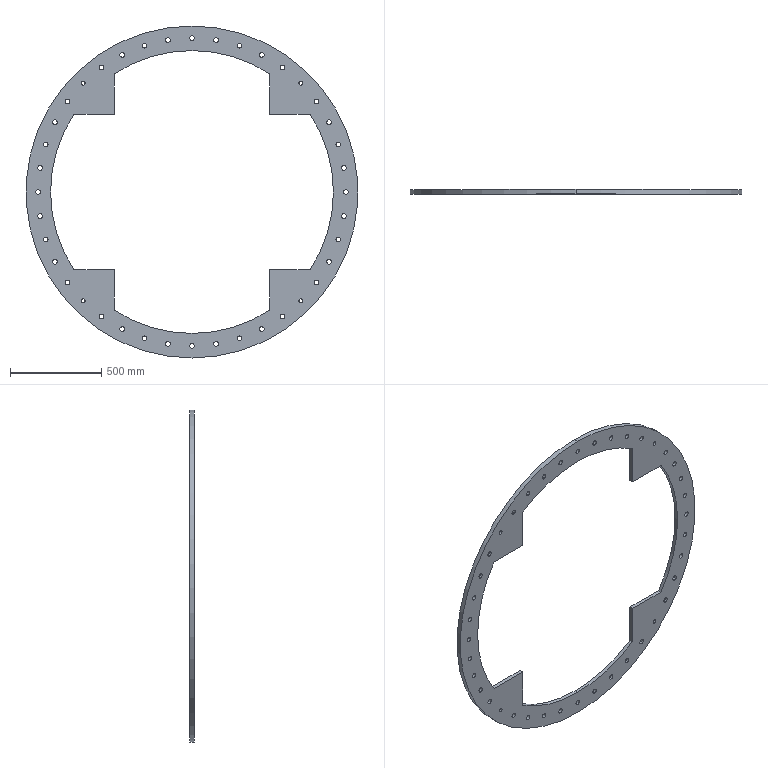Part | SolidWorks | features HoleWzd 2, CirPattern 1, Extrusion 1, ICE 1 | 1 solid | 100 faces | box 1820 x 25 x 1820 mm | volume 17265104 mm3 | cylinder 89 | plane 11 | commonest cylinder face diameters 26 x72 21 x8 1550 x5 1740 x2 1820 x2